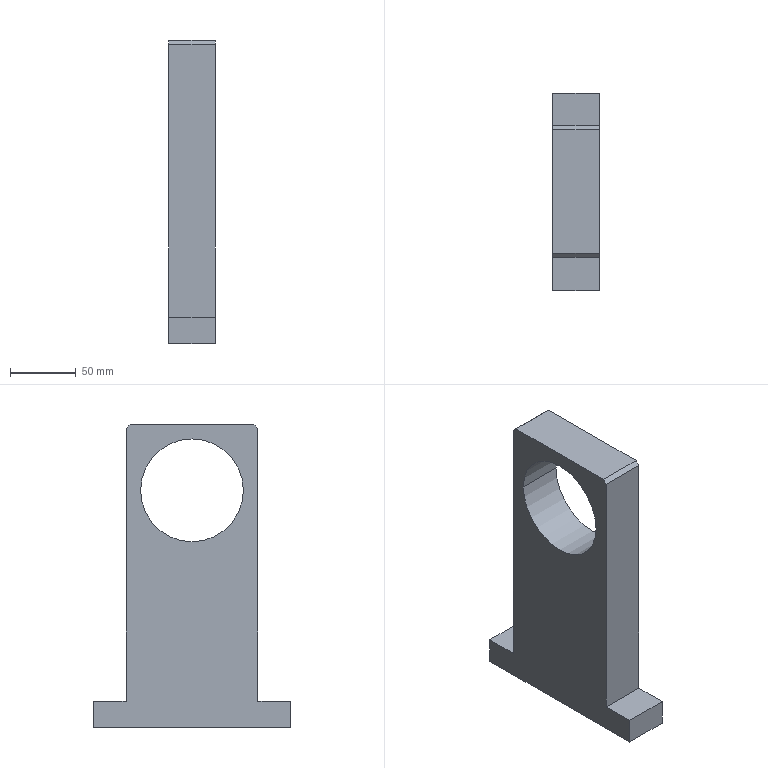Part | NX | features 0006 2 | 1 solid | 14 faces | box 35 x 150 x 230 mm | volume 672442 mm3 | plane 12 | cylinder 2 | commonest cylinder face diameters 78 x2
STEP:
#1=CARTESIAN_POINT('',(-203.3,-80.,-820.129));
#2=VERTEX_POINT('',#1);
#3=CARTESIAN_POINT('',(-203.3,-158.,-820.129));
#4=VERTEX_POINT('',#3);
#5=CARTESIAN_POINT('',(-203.3,-119.,-820.129));
#6=DIRECTION('',(1.,0.,0.));
#7=DIRECTION('',(0.,1.,0.));
#8=AXIS2_PLACEMENT_3D('',#5,#6,#7);
#9=CIRCLE('',#8,39.);
#10=EDGE_CURVE('',#2,#4,#9,.T.);
#11=ORIENTED_EDGE('',*,*,#10,.F.);
#12=CARTESIAN_POINT('',(-168.3,-80.,-820.129));
#13=VERTEX_POINT('',#12);
#14=CARTESIAN_POINT('',(-168.3,-80.,-820.129));
#15=DIRECTION('',(-1.,0.,0.));
#16=VECTOR('',#15,1000.);
#17=LINE('',#14,#16);
#18=EDGE_CURVE('',#13,#2,#17,.T.);
#19=ORIENTED_EDGE('',*,*,#18,.F.);
#20=CARTESIAN_POINT('',(-168.3,-158.,-820.129));
#21=VERTEX_POINT('',#20);
#22=CARTESIAN_POINT('',(-168.3,-119.,-820.129));
#23=DIRECTION('',(-1.,0.,0.));
#24=DIRECTION('',(0.,-1.,0.));
#25=AXIS2_PLACEMENT_3D('',#22,#23,#24);
#26=CIRCLE('',#25,39.);
#27=EDGE_CURVE('',#21,#13,#26,.T.);
#28=ORIENTED_EDGE('',*,*,#27,.F.);
#29=CARTESIAN_POINT('',(-168.3,-158.,-820.129));
#30=DIRECTION('',(-1.,0.,0.));
#31=VECTOR('',#30,1000.);
#32=LINE('',#29,#31);
#33=EDGE_CURVE('',#4,#21,#32,.F.);
#34=ORIENTED_EDGE('',*,*,#33,.F.);
#35=EDGE_LOOP('',(#11,#19,#28,#34));
#36=FACE_BOUND('',#35,.T.);
#37=CARTESIAN_POINT('',(-203.3,-119.,-820.129));
#38=DIRECTION('',(1.,0.,0.));
#39=DIRECTION('',(0.,1.,0.));
#40=AXIS2_PLACEMENT_3D('',#37,#38,#39);
#41=CYLINDRICAL_SURFACE('',#40,39.);
#42=ADVANCED_FACE('',(#36),#41,.F.);
#43=ORIENTED_EDGE('',*,*,#33,.T.);
#44=CARTESIAN_POINT('',(-168.3,-119.,-820.129));
#45=DIRECTION('',(-1.,0.,0.));
#46=DIRECTION('',(0.,1.,0.));
#47=AXIS2_PLACEMENT_3D('',#44,#45,#46);
#48=CIRCLE('',#47,39.);
#49=EDGE_CURVE('',#13,#21,#48,.T.);
#50=ORIENTED_EDGE('',*,*,#49,.F.);
#51=ORIENTED_EDGE('',*,*,#18,.T.);
#52=CARTESIAN_POINT('',(-203.3,-119.,-820.129));
#53=DIRECTION('',(1.,0.,0.));
#54=DIRECTION('',(0.,-1.,0.));
#55=AXIS2_PLACEMENT_3D('',#52,#53,#54);
#56=CIRCLE('',#55,39.);
#57=EDGE_CURVE('',#4,#2,#56,.T.);
#58=ORIENTED_EDGE('',*,*,#57,.F.);
#59=EDGE_LOOP('',(#43,#50,#51,#58));
#60=FACE_BOUND('',#59,.T.);
#61=CARTESIAN_POINT('',(-203.3,-119.,-820.129));
#62=DIRECTION('',(1.,0.,0.));
#63=DIRECTION('',(0.,1.,0.));
#64=AXIS2_PLACEMENT_3D('',#61,#62,#63);
#65=CYLINDRICAL_SURFACE('',#64,39.);
#66=ADVANCED_FACE('',(#60),#65,.F.);
#67=CARTESIAN_POINT('',(-168.3,-44.,-980.129));
#68=VERTEX_POINT('',#67);
#69=CARTESIAN_POINT('',(-203.3,-44.,-980.129));
#70=VERTEX_POINT('',#69);
#71=CARTESIAN_POINT('',(-168.3,-44.,-980.129));
#72=DIRECTION('',(-1.,0.,0.));
#73=VECTOR('',#72,1000.);
#74=LINE('',#71,#73);
#75=EDGE_CURVE('',#68,#70,#74,.T.);
#76=ORIENTED_EDGE('',*,*,#75,.T.);
#77=CARTESIAN_POINT('',(-203.3,-69.,-980.129));
#78=VERTEX_POINT('',#77);
#79=CARTESIAN_POINT('',(-203.3,-44.,-980.129));
#80=DIRECTION('',(0.,-1.,0.));
#81=VECTOR('',#80,1000.);
#82=LINE('',#79,#81);
#83=EDGE_CURVE('',#70,#78,#82,.T.);
#84=ORIENTED_EDGE('',*,*,#83,.T.);
#85=CARTESIAN_POINT('',(-168.3,-69.,-980.129));
#86=VERTEX_POINT('',#85);
#87=CARTESIAN_POINT('',(-168.3,-69.,-980.129));
#88=DIRECTION('',(-1.,0.,0.));
#89=VECTOR('',#88,1000.);
#90=LINE('',#87,#89);
#91=EDGE_CURVE('',#86,#78,#90,.T.);
#92=ORIENTED_EDGE('',*,*,#91,.F.);
#93=CARTESIAN_POINT('',(-168.3,-44.,-980.129));
#94=DIRECTION('',(0.,-1.,0.));
#95=VECTOR('',#94,1000.);
#96=LINE('',#93,#95);
#97=EDGE_CURVE('',#68,#86,#96,.T.);
#98=ORIENTED_EDGE('',*,*,#97,.F.);
#99=EDGE_LOOP('',(#76,#84,#92,#98));
#100=FACE_BOUND('',#99,.T.);
#101=CARTESIAN_POINT('',(-203.3,-69.,-980.129));
#102=DIRECTION('',(0.,0.,-1.));
#103=DIRECTION('',(0.,-1.,0.));
#104=AXIS2_PLACEMENT_3D('',#101,#102,#103);
#105=PLANE('',#104);
#106=ADVANCED_FACE('',(#100),#105,.F.);
#107=CARTESIAN_POINT('',(-203.3,-72.,-770.129));
#108=VERTEX_POINT('',#107);
#109=CARTESIAN_POINT('',(-168.3,-72.,-770.129));
#110=VERTEX_POINT('',#109);
#111=CARTESIAN_POINT('',(-203.3,-72.,-770.129));
#112=DIRECTION('',(1.,0.,0.));
#113=VECTOR('',#112,1000.);
#114=LINE('',#111,#113);
#115=EDGE_CURVE('',#108,#110,#114,.T.);
#116=ORIENTED_EDGE('',*,*,#115,.T.);
#117=CARTESIAN_POINT('',(-168.3,-69.,-773.129));
#118=VERTEX_POINT('',#117);
#119=CARTESIAN_POINT('',(-168.3,-69.,-773.129));
#120=DIRECTION('',(0.,-0.7071,0.7071));
#121=VECTOR('',#120,1000.);
#122=LINE('',#119,#121);
#123=EDGE_CURVE('',#118,#110,#122,.T.);
#124=ORIENTED_EDGE('',*,*,#123,.F.);
#125=CARTESIAN_POINT('',(-203.3,-69.,-773.129));
#126=VERTEX_POINT('',#125);
#127=CARTESIAN_POINT('',(-168.3,-69.,-773.129));
#128=DIRECTION('',(-1.,0.,0.));
#129=VECTOR('',#128,1000.);
#130=LINE('',#127,#129);
#131=EDGE_CURVE('',#118,#126,#130,.T.);
#132=ORIENTED_EDGE('',*,*,#131,.T.);
#133=CARTESIAN_POINT('',(-203.3,-72.,-770.129));
#134=DIRECTION('',(0.,0.7071,-0.7071));
#135=VECTOR('',#134,1000.);
#136=LINE('',#133,#135);
#137=EDGE_CURVE('',#108,#126,#136,.T.);
#138=ORIENTED_EDGE('',*,*,#137,.F.);
#139=EDGE_LOOP('',(#116,#124,#132,#138));
#140=FACE_BOUND('',#139,.T.);
#141=CARTESIAN_POINT('',(-203.3,-69.,-773.129));
#142=DIRECTION('',(0.,-0.7071,-0.7071));
#143=DIRECTION('',(1.,0.,0.));
#144=AXIS2_PLACEMENT_3D('',#141,#142,#143);
#145=PLANE('',#144);
#146=ADVANCED_FACE('',(#140),#145,.F.);
#147=CARTESIAN_POINT('',(-168.3,-194.,-1000.129));
#148=VERTEX_POINT('',#147);
#149=CARTESIAN_POINT('',(-203.3,-194.,-1000.129));
#150=VERTEX_POINT('',#149);
#151=CARTESIAN_POINT('',(-168.3,-194.,-1000.129));
#152=DIRECTION('',(-1.,0.,0.));
#153=VECTOR('',#152,1000.);
#154=LINE('',#151,#153);
#155=EDGE_CURVE('',#148,#150,#154,.T.);
#156=ORIENTED_EDGE('',*,*,#155,.T.);
#157=CARTESIAN_POINT('',(-203.3,-44.,-1000.129));
#158=VERTEX_POINT('',#157);
#159=CARTESIAN_POINT('',(-203.3,-194.,-1000.129));
#160=DIRECTION('',(0.,1.,0.));
#161=VECTOR('',#160,1000.);
#162=LINE('',#159,#161);
#163=EDGE_CURVE('',#150,#158,#162,.T.);
#164=ORIENTED_EDGE('',*,*,#163,.T.);
#165=CARTESIAN_POINT('',(-168.3,-44.,-1000.129));
#166=VERTEX_POINT('',#165);
#167=CARTESIAN_POINT('',(-168.3,-44.,-1000.129));
#168=DIRECTION('',(-1.,0.,0.));
#169=VECTOR('',#168,1000.);
#170=LINE('',#167,#169);
#171=EDGE_CURVE('',#166,#158,#170,.T.);
#172=ORIENTED_EDGE('',*,*,#171,.F.);
#173=CARTESIAN_POINT('',(-168.3,-194.,-1000.129));
#174=DIRECTION('',(0.,1.,0.));
#175=VECTOR('',#174,1000.);
#176=LINE('',#173,#175);
#177=EDGE_CURVE('',#148,#166,#176,.T.);
#178=ORIENTED_EDGE('',*,*,#177,.F.);
#179=EDGE_LOOP('',(#156,#164,#172,#178));
#180=FACE_BOUND('',#179,.T.);
#181=CARTESIAN_POINT('',(-203.3,-194.,-1000.129));
#182=DIRECTION('',(0.,0.,1.));
#183=DIRECTION('',(0.,1.,0.));
#184=AXIS2_PLACEMENT_3D('',#181,#182,#183);
#185=PLANE('',#184);
#186=ADVANCED_FACE('',(#180),#185,.F.);
#187=CARTESIAN_POINT('',(-168.3,-194.,-980.129));
#188=VERTEX_POINT('',#187);
#189=CARTESIAN_POINT('',(-203.3,-194.,-980.129));
#190=VERTEX_POINT('',#189);
#191=CARTESIAN_POINT('',(-168.3,-194.,-980.129));
#192=DIRECTION('',(-1.,0.,0.));
#193=VECTOR('',#192,1000.);
#194=LINE('',#191,#193);
#195=EDGE_CURVE('',#188,#190,#194,.T.);
#196=ORIENTED_EDGE('',*,*,#195,.T.);
#197=CARTESIAN_POINT('',(-203.3,-194.,-980.129));
#198=DIRECTION('',(0.,0.,-1.));
#199=VECTOR('',#198,1000.);
#200=LINE('',#197,#199);
#201=EDGE_CURVE('',#190,#150,#200,.T.);
#202=ORIENTED_EDGE('',*,*,#201,.T.);
#203=ORIENTED_EDGE('',*,*,#155,.F.);
#204=CARTESIAN_POINT('',(-168.3,-194.,-980.129));
#205=DIRECTION('',(0.,0.,-1.));
#206=VECTOR('',#205,1000.);
#207=LINE('',#204,#206);
#208=EDGE_CURVE('',#188,#148,#207,.T.);
#209=ORIENTED_EDGE('',*,*,#208,.F.);
#210=EDGE_LOOP('',(#196,#202,#203,#209));
#211=FACE_BOUND('',#210,.T.);
#212=CARTESIAN_POINT('',(-203.3,-194.,-980.129));
#213=DIRECTION('',(0.,1.,0.));
#214=DIRECTION('',(0.,0.,-1.));
#215=AXIS2_PLACEMENT_3D('',#212,#213,#214);
#216=PLANE('',#215);
#217=ADVANCED_FACE('',(#211),#216,.F.);
#218=CARTESIAN_POINT('',(-168.3,-169.,-980.129));
#219=VERTEX_POINT('',#218);
#220=CARTESIAN_POINT('',(-203.3,-169.,-980.129));
#221=VERTEX_POINT('',#220);
#222=CARTESIAN_POINT('',(-168.3,-169.,-980.129));
#223=DIRECTION('',(-1.,0.,0.));
#224=VECTOR('',#223,1000.);
#225=LINE('',#222,#224);
#226=EDGE_CURVE('',#219,#221,#225,.T.);
#227=ORIENTED_EDGE('',*,*,#226,.T.);
#228=CARTESIAN_POINT('',(-203.3,-169.,-980.129));
#229=DIRECTION('',(0.,-1.,0.));
#230=VECTOR('',#229,1000.);
#231=LINE('',#228,#230);
#232=EDGE_CURVE('',#221,#190,#231,.T.);
#233=ORIENTED_EDGE('',*,*,#232,.T.);
#234=ORIENTED_EDGE('',*,*,#195,.F.);
#235=CARTESIAN_POINT('',(-168.3,-169.,-980.129));
#236=DIRECTION('',(0.,-1.,0.));
#237=VECTOR('',#236,1000.);
#238=LINE('',#235,#237);
#239=EDGE_CURVE('',#219,#188,#238,.T.);
#240=ORIENTED_EDGE('',*,*,#239,.F.);
#241=EDGE_LOOP('',(#227,#233,#234,#240));
#242=FACE_BOUND('',#241,.T.);
#243=CARTESIAN_POINT('',(-203.3,-169.,-980.129));
#244=DIRECTION('',(0.,0.,-1.));
#245=DIRECTION('',(0.,-1.,0.));
#246=AXIS2_PLACEMENT_3D('',#243,#244,#245);
#247=PLANE('',#246);
#248=ADVANCED_FACE('',(#242),#247,.F.);
#249=CARTESIAN_POINT('',(-203.3,-169.,-773.129));
#250=VERTEX_POINT('',#249);
#251=CARTESIAN_POINT('',(-168.3,-169.,-773.129));
#252=VERTEX_POINT('',#251);
#253=CARTESIAN_POINT('',(-203.3,-169.,-773.129));
#254=DIRECTION('',(1.,0.,0.));
#255=VECTOR('',#254,1000.);
#256=LINE('',#253,#255);
#257=EDGE_CURVE('',#250,#252,#256,.T.);
#258=ORIENTED_EDGE('',*,*,#257,.F.);
#259=CARTESIAN_POINT('',(-203.3,-169.,-773.129));
#260=DIRECTION('',(0.,0.,-1.));
#261=VECTOR('',#260,1000.);
#262=LINE('',#259,#261);
#263=EDGE_CURVE('',#250,#221,#262,.T.);
#264=ORIENTED_EDGE('',*,*,#263,.T.);
#265=ORIENTED_EDGE('',*,*,#226,.F.);
#266=CARTESIAN_POINT('',(-168.3,-169.,-773.129));
#267=DIRECTION('',(0.,0.,-1.));
#268=VECTOR('',#267,1000.);
#269=LINE('',#266,#268);
#270=EDGE_CURVE('',#252,#219,#269,.T.);
#271=ORIENTED_EDGE('',*,*,#270,.F.);
#272=EDGE_LOOP('',(#258,#264,#265,#271));
#273=FACE_BOUND('',#272,.T.);
#274=CARTESIAN_POINT('',(-203.3,-169.,-770.129));
#275=DIRECTION('',(0.,1.,0.));
#276=DIRECTION('',(0.,0.,-1.));
#277=AXIS2_PLACEMENT_3D('',#274,#275,#276);
#278=PLANE('',#277);
#279=ADVANCED_FACE('',(#273),#278,.F.);
#280=ORIENTED_EDGE('',*,*,#257,.T.);
#281=CARTESIAN_POINT('',(-168.3,-166.,-770.129));
#282=VERTEX_POINT('',#281);
#283=CARTESIAN_POINT('',(-168.3,-166.,-770.129));
#284=DIRECTION('',(0.,-0.7071,-0.7071));
#285=VECTOR('',#284,1000.);
#286=LINE('',#283,#285);
#287=EDGE_CURVE('',#282,#252,#286,.T.);
#288=ORIENTED_EDGE('',*,*,#287,.F.);
#289=CARTESIAN_POINT('',(-203.3,-166.,-770.129));
#290=VERTEX_POINT('',#289);
#291=CARTESIAN_POINT('',(-168.3,-166.,-770.129));
#292=DIRECTION('',(-1.,0.,0.));
#293=VECTOR('',#292,1000.);
#294=LINE('',#291,#293);
#295=EDGE_CURVE('',#282,#290,#294,.T.);
#296=ORIENTED_EDGE('',*,*,#295,.T.);
#297=CARTESIAN_POINT('',(-203.3,-169.,-773.129));
#298=DIRECTION('',(0.,0.7071,0.7071));
#299=VECTOR('',#298,1000.);
#300=LINE('',#297,#299);
#301=EDGE_CURVE('',#250,#290,#300,.T.);
#302=ORIENTED_EDGE('',*,*,#301,.F.);
#303=EDGE_LOOP('',(#280,#288,#296,#302));
#304=FACE_BOUND('',#303,.T.);
#305=CARTESIAN_POINT('',(-203.3,-166.,-770.129));
#306=DIRECTION('',(0.,0.7071,-0.7071));
#307=DIRECTION('',(1.,0.,0.));
#308=AXIS2_PLACEMENT_3D('',#305,#306,#307);
#309=PLANE('',#308);
#310=ADVANCED_FACE('',(#304),#309,.F.);
#311=ORIENTED_EDGE('',*,*,#115,.F.);
#312=CARTESIAN_POINT('',(-203.3,-72.,-770.129));
#313=DIRECTION('',(0.,-1.,0.));
#314=VECTOR('',#313,1000.);
#315=LINE('',#312,#314);
#316=EDGE_CURVE('',#108,#290,#315,.T.);
#317=ORIENTED_EDGE('',*,*,#316,.T.);
#318=ORIENTED_EDGE('',*,*,#295,.F.);
#319=CARTESIAN_POINT('',(-168.3,-72.,-770.129));
#320=DIRECTION('',(0.,-1.,0.));
#321=VECTOR('',#320,1000.);
#322=LINE('',#319,#321);
#323=EDGE_CURVE('',#110,#282,#322,.T.);
#324=ORIENTED_EDGE('',*,*,#323,.F.);
#325=EDGE_LOOP('',(#311,#317,#318,#324));
#326=FACE_BOUND('',#325,.T.);
#327=CARTESIAN_POINT('',(-203.3,-69.,-770.129));
#328=DIRECTION('',(0.,0.,-1.));
#329=DIRECTION('',(0.,-1.,0.));
#330=AXIS2_PLACEMENT_3D('',#327,#328,#329);
#331=PLANE('',#330);
#332=ADVANCED_FACE('',(#326),#331,.F.);
#333=ORIENTED_EDGE('',*,*,#10,.T.);
#334=ORIENTED_EDGE('',*,*,#57,.T.);
#335=EDGE_LOOP('',(#333,#334));
#336=FACE_BOUND('',#335,.T.);
#337=ORIENTED_EDGE('',*,*,#137,.T.);
#338=CARTESIAN_POINT('',(-203.3,-69.,-980.129));
#339=DIRECTION('',(0.,0.,1.));
#340=VECTOR('',#339,1000.);
#341=LINE('',#338,#340);
#342=EDGE_CURVE('',#78,#126,#341,.T.);
#343=ORIENTED_EDGE('',*,*,#342,.F.);
#344=ORIENTED_EDGE('',*,*,#83,.F.);
#345=CARTESIAN_POINT('',(-203.3,-44.,-1000.129));
#346=DIRECTION('',(0.,0.,1.));
#347=VECTOR('',#346,1000.);
#348=LINE('',#345,#347);
#349=EDGE_CURVE('',#158,#70,#348,.T.);
#350=ORIENTED_EDGE('',*,*,#349,.F.);
#351=ORIENTED_EDGE('',*,*,#163,.F.);
#352=ORIENTED_EDGE('',*,*,#201,.F.);
#353=ORIENTED_EDGE('',*,*,#232,.F.);
#354=ORIENTED_EDGE('',*,*,#263,.F.);
#355=ORIENTED_EDGE('',*,*,#301,.T.);
#356=ORIENTED_EDGE('',*,*,#316,.F.);
#357=EDGE_LOOP('',(#337,#343,#344,#350,#351,#352,#353,#354,#355,#356));
#358=FACE_BOUND('',#357,.T.);
#359=CARTESIAN_POINT('',(-203.3,-119.,-1000.129));
#360=DIRECTION('',(-1.,0.,0.));
#361=DIRECTION('',(0.,-1.,0.));
#362=AXIS2_PLACEMENT_3D('',#359,#360,#361);
#363=PLANE('',#362);
#364=ADVANCED_FACE('',(#336,#358),#363,.T.);
#365=ORIENTED_EDGE('',*,*,#131,.F.);
#366=CARTESIAN_POINT('',(-168.3,-69.,-980.129));
#367=DIRECTION('',(0.,0.,1.));
#368=VECTOR('',#367,1000.);
#369=LINE('',#366,#368);
#370=EDGE_CURVE('',#86,#118,#369,.T.);
#371=ORIENTED_EDGE('',*,*,#370,.F.);
#372=ORIENTED_EDGE('',*,*,#91,.T.);
#373=ORIENTED_EDGE('',*,*,#342,.T.);
#374=EDGE_LOOP('',(#365,#371,#372,#373));
#375=FACE_BOUND('',#374,.T.);
#376=CARTESIAN_POINT('',(-203.3,-69.,-770.129));
#377=DIRECTION('',(0.,-1.,0.));
#378=DIRECTION('',(0.,0.,1.));
#379=AXIS2_PLACEMENT_3D('',#376,#377,#378);
#380=PLANE('',#379);
#381=ADVANCED_FACE('',(#375),#380,.F.);
#382=ORIENTED_EDGE('',*,*,#27,.T.);
#383=ORIENTED_EDGE('',*,*,#49,.T.);
#384=EDGE_LOOP('',(#382,#383));
#385=FACE_BOUND('',#384,.T.);
#386=ORIENTED_EDGE('',*,*,#123,.T.);
#387=ORIENTED_EDGE('',*,*,#323,.T.);
#388=ORIENTED_EDGE('',*,*,#287,.T.);
#389=ORIENTED_EDGE('',*,*,#270,.T.);
#390=ORIENTED_EDGE('',*,*,#239,.T.);
#391=ORIENTED_EDGE('',*,*,#208,.T.);
#392=ORIENTED_EDGE('',*,*,#177,.T.);
#393=CARTESIAN_POINT('',(-168.3,-44.,-1000.129));
#394=DIRECTION('',(0.,0.,1.));
#395=VECTOR('',#394,1000.);
#396=LINE('',#393,#395);
#397=EDGE_CURVE('',#166,#68,#396,.T.);
#398=ORIENTED_EDGE('',*,*,#397,.T.);
#399=ORIENTED_EDGE('',*,*,#97,.T.);
#400=ORIENTED_EDGE('',*,*,#370,.T.);
#401=EDGE_LOOP('',(#386,#387,#388,#389,#390,#391,#392,#398,#399,#400));
#402=FACE_BOUND('',#401,.T.);
#403=CARTESIAN_POINT('',(-168.3,-119.,-1000.129));
#404=DIRECTION('',(-1.,0.,0.));
#405=DIRECTION('',(0.,-1.,0.));
#406=AXIS2_PLACEMENT_3D('',#403,#404,#405);
#407=PLANE('',#406);
#408=ADVANCED_FACE('',(#385,#402),#407,.F.);
#409=ORIENTED_EDGE('',*,*,#171,.T.);
#410=ORIENTED_EDGE('',*,*,#349,.T.);
#411=ORIENTED_EDGE('',*,*,#75,.F.);
#412=ORIENTED_EDGE('',*,*,#397,.F.);
#413=EDGE_LOOP('',(#409,#410,#411,#412));
#414=FACE_BOUND('',#413,.T.);
#415=CARTESIAN_POINT('',(-203.3,-44.,-980.129));
#416=DIRECTION('',(0.,-1.,0.));
#417=DIRECTION('',(0.,0.,1.));
#418=AXIS2_PLACEMENT_3D('',#415,#416,#417);
#419=PLANE('',#418);
#420=ADVANCED_FACE('',(#414),#419,.F.);
#421=CLOSED_SHELL('',(#42,#66,#106,#146,#186,#217,#248,#279,#310,#332,#364,#381,#408,#420));
#422=MANIFOLD_SOLID_BREP('',#421);
#423=(LENGTH_UNIT()NAMED_UNIT(*)SI_UNIT(.MILLI.,.METRE.));
#424=UNCERTAINTY_MEASURE_WITH_UNIT(LENGTH_MEASURE(0.00001),#423,'','');
#425=(NAMED_UNIT(*)PLANE_ANGLE_UNIT()SI_UNIT($,.RADIAN.));
#426=(NAMED_UNIT(*)SI_UNIT($,.STERADIAN.)SOLID_ANGLE_UNIT());
#427=(GEOMETRIC_REPRESENTATION_CONTEXT(3)GLOBAL_UNCERTAINTY_ASSIGNED_CONTEXT((#424))GLOBAL_UNIT_ASSIGNED_CONTEXT((#423,#425,#426))REPRESENTATION_CONTEXT('',''));
#428=ADVANCED_BREP_SHAPE_REPRESENTATION('',(#422),#427);